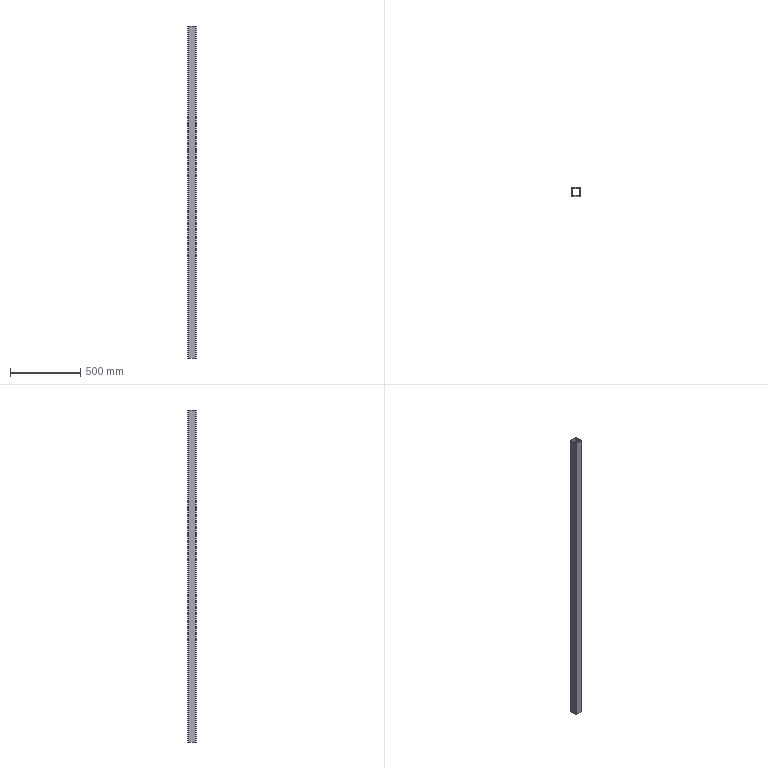Part | STEP file | 750078154 | 1 solid | 18 faces | box 60 x 60 x 2360 mm | volume 2049733 mm3 | plane 10 | cylinder 8 | commonest cylinder face diameters 4 x4 12 x4
STEP:
#1=CARTESIAN_POINT('',(-26.,24.,2360.));
#2=VERTEX_POINT('',#1);
#3=CARTESIAN_POINT('',(-26.,24.,0.));
#4=VERTEX_POINT('',#3);
#5=CARTESIAN_POINT('',(-26.,24.,2360.));
#6=DIRECTION('',(0.,0.,-1.));
#7=VECTOR('',#6,1000.);
#8=LINE('',#5,#7);
#9=EDGE_CURVE('',#2,#4,#8,.T.);
#10=ORIENTED_EDGE('',*,*,#9,.F.);
#11=CARTESIAN_POINT('',(-26.,-24.,2360.));
#12=VERTEX_POINT('',#11);
#13=CARTESIAN_POINT('',(-26.,-24.,2360.));
#14=DIRECTION('',(0.,1.,0.));
#15=VECTOR('',#14,1000.);
#16=LINE('',#13,#15);
#17=EDGE_CURVE('',#12,#2,#16,.T.);
#18=ORIENTED_EDGE('',*,*,#17,.F.);
#19=CARTESIAN_POINT('',(-26.,-24.,0.));
#20=VERTEX_POINT('',#19);
#21=CARTESIAN_POINT('',(-26.,-24.,2360.));
#22=DIRECTION('',(0.,0.,1.));
#23=VECTOR('',#22,1000.);
#24=LINE('',#21,#23);
#25=EDGE_CURVE('',#20,#12,#24,.T.);
#26=ORIENTED_EDGE('',*,*,#25,.F.);
#27=CARTESIAN_POINT('',(-26.,-24.,0.));
#28=DIRECTION('',(0.,-1.,0.));
#29=VECTOR('',#28,1000.);
#30=LINE('',#27,#29);
#31=EDGE_CURVE('',#4,#20,#30,.T.);
#32=ORIENTED_EDGE('',*,*,#31,.F.);
#33=EDGE_LOOP('',(#10,#18,#26,#32));
#34=FACE_OUTER_BOUND('',#33,.T.);
#35=CARTESIAN_POINT('',(-26.,-24.,2360.));
#36=DIRECTION('',(-1.,0.,0.));
#37=DIRECTION('',(0.,-1.,0.));
#38=AXIS2_PLACEMENT_3D('',#35,#36,#37);
#39=PLANE('',#38);
#40=ADVANCED_FACE('',(#34),#39,.F.);
#41=CARTESIAN_POINT('',(26.,24.,0.));
#42=VERTEX_POINT('',#41);
#43=CARTESIAN_POINT('',(24.,26.,0.));
#44=VERTEX_POINT('',#43);
#45=CARTESIAN_POINT('',(24.,24.,0.));
#46=DIRECTION('',(0.,0.,1.));
#47=DIRECTION('',(-1.,0.,0.));
#48=AXIS2_PLACEMENT_3D('',#45,#46,#47);
#49=CIRCLE('',#48,2.);
#50=EDGE_CURVE('',#42,#44,#49,.T.);
#51=ORIENTED_EDGE('',*,*,#50,.T.);
#52=CARTESIAN_POINT('',(-24.,26.,0.));
#53=VERTEX_POINT('',#52);
#54=CARTESIAN_POINT('',(24.,26.,0.));
#55=DIRECTION('',(-1.,0.,0.));
#56=VECTOR('',#55,1000.);
#57=LINE('',#54,#56);
#58=EDGE_CURVE('',#44,#53,#57,.T.);
#59=ORIENTED_EDGE('',*,*,#58,.T.);
#60=CARTESIAN_POINT('',(-24.,24.,0.));
#61=DIRECTION('',(0.,0.,1.));
#62=DIRECTION('',(-1.,0.,0.));
#63=AXIS2_PLACEMENT_3D('',#60,#61,#62);
#64=CIRCLE('',#63,2.);
#65=EDGE_CURVE('',#53,#4,#64,.T.);
#66=ORIENTED_EDGE('',*,*,#65,.T.);
#67=ORIENTED_EDGE('',*,*,#31,.T.);
#68=CARTESIAN_POINT('',(-24.,-26.,0.));
#69=VERTEX_POINT('',#68);
#70=CARTESIAN_POINT('',(-24.,-24.,0.));
#71=DIRECTION('',(0.,0.,1.));
#72=DIRECTION('',(-1.,0.,0.));
#73=AXIS2_PLACEMENT_3D('',#70,#71,#72);
#74=CIRCLE('',#73,2.);
#75=EDGE_CURVE('',#20,#69,#74,.T.);
#76=ORIENTED_EDGE('',*,*,#75,.T.);
#77=CARTESIAN_POINT('',(24.,-26.,0.));
#78=VERTEX_POINT('',#77);
#79=CARTESIAN_POINT('',(24.,-26.,0.));
#80=DIRECTION('',(1.,0.,0.));
#81=VECTOR('',#80,1000.);
#82=LINE('',#79,#81);
#83=EDGE_CURVE('',#69,#78,#82,.T.);
#84=ORIENTED_EDGE('',*,*,#83,.T.);
#85=CARTESIAN_POINT('',(26.,-24.,0.));
#86=VERTEX_POINT('',#85);
#87=CARTESIAN_POINT('',(24.,-24.,0.));
#88=DIRECTION('',(0.,0.,1.));
#89=DIRECTION('',(-1.,0.,0.));
#90=AXIS2_PLACEMENT_3D('',#87,#88,#89);
#91=CIRCLE('',#90,2.);
#92=EDGE_CURVE('',#78,#86,#91,.T.);
#93=ORIENTED_EDGE('',*,*,#92,.T.);
#94=CARTESIAN_POINT('',(26.,-24.,0.));
#95=DIRECTION('',(0.,1.,0.));
#96=VECTOR('',#95,1000.);
#97=LINE('',#94,#96);
#98=EDGE_CURVE('',#86,#42,#97,.T.);
#99=ORIENTED_EDGE('',*,*,#98,.T.);
#100=EDGE_LOOP('',(#51,#59,#66,#67,#76,#84,#93,#99));
#101=FACE_BOUND('',#100,.T.);
#102=CARTESIAN_POINT('',(-24.,30.,0.));
#103=VERTEX_POINT('',#102);
#104=CARTESIAN_POINT('',(24.,30.,0.));
#105=VERTEX_POINT('',#104);
#106=CARTESIAN_POINT('',(24.,30.,0.));
#107=DIRECTION('',(1.,0.,0.));
#108=VECTOR('',#107,1000.);
#109=LINE('',#106,#108);
#110=EDGE_CURVE('',#103,#105,#109,.T.);
#111=ORIENTED_EDGE('',*,*,#110,.T.);
#112=CARTESIAN_POINT('',(30.,24.,0.));
#113=VERTEX_POINT('',#112);
#114=CARTESIAN_POINT('',(24.,24.,0.));
#115=DIRECTION('',(0.,0.,-1.));
#116=DIRECTION('',(-1.,0.,0.));
#117=AXIS2_PLACEMENT_3D('',#114,#115,#116);
#118=CIRCLE('',#117,6.);
#119=EDGE_CURVE('',#105,#113,#118,.T.);
#120=ORIENTED_EDGE('',*,*,#119,.T.);
#121=CARTESIAN_POINT('',(30.,-24.,0.));
#122=VERTEX_POINT('',#121);
#123=CARTESIAN_POINT('',(30.,-24.,0.));
#124=DIRECTION('',(0.,-1.,0.));
#125=VECTOR('',#124,1000.);
#126=LINE('',#123,#125);
#127=EDGE_CURVE('',#113,#122,#126,.T.);
#128=ORIENTED_EDGE('',*,*,#127,.T.);
#129=CARTESIAN_POINT('',(24.,-30.,0.));
#130=VERTEX_POINT('',#129);
#131=CARTESIAN_POINT('',(24.,-24.,0.));
#132=DIRECTION('',(0.,0.,-1.));
#133=DIRECTION('',(-1.,0.,0.));
#134=AXIS2_PLACEMENT_3D('',#131,#132,#133);
#135=CIRCLE('',#134,6.);
#136=EDGE_CURVE('',#122,#130,#135,.T.);
#137=ORIENTED_EDGE('',*,*,#136,.T.);
#138=CARTESIAN_POINT('',(-24.,-30.,0.));
#139=VERTEX_POINT('',#138);
#140=CARTESIAN_POINT('',(24.,-30.,0.));
#141=DIRECTION('',(-1.,0.,0.));
#142=VECTOR('',#141,1000.);
#143=LINE('',#140,#142);
#144=EDGE_CURVE('',#130,#139,#143,.T.);
#145=ORIENTED_EDGE('',*,*,#144,.T.);
#146=CARTESIAN_POINT('',(-30.,-24.,0.));
#147=VERTEX_POINT('',#146);
#148=CARTESIAN_POINT('',(-24.,-24.,0.));
#149=DIRECTION('',(0.,0.,-1.));
#150=DIRECTION('',(-1.,0.,0.));
#151=AXIS2_PLACEMENT_3D('',#148,#149,#150);
#152=CIRCLE('',#151,6.);
#153=EDGE_CURVE('',#139,#147,#152,.T.);
#154=ORIENTED_EDGE('',*,*,#153,.T.);
#155=CARTESIAN_POINT('',(-30.,24.,0.));
#156=VERTEX_POINT('',#155);
#157=CARTESIAN_POINT('',(-30.,-24.,0.));
#158=DIRECTION('',(0.,1.,0.));
#159=VECTOR('',#158,1000.);
#160=LINE('',#157,#159);
#161=EDGE_CURVE('',#147,#156,#160,.T.);
#162=ORIENTED_EDGE('',*,*,#161,.T.);
#163=CARTESIAN_POINT('',(-24.,24.,0.));
#164=DIRECTION('',(0.,0.,-1.));
#165=DIRECTION('',(-1.,0.,0.));
#166=AXIS2_PLACEMENT_3D('',#163,#164,#165);
#167=CIRCLE('',#166,6.);
#168=EDGE_CURVE('',#156,#103,#167,.T.);
#169=ORIENTED_EDGE('',*,*,#168,.T.);
#170=EDGE_LOOP('',(#111,#120,#128,#137,#145,#154,#162,#169));
#171=FACE_OUTER_BOUND('',#170,.T.);
#172=CARTESIAN_POINT('',(24.,-24.,0.));
#173=DIRECTION('',(0.,0.,-1.));
#174=DIRECTION('',(-1.,0.,0.));
#175=AXIS2_PLACEMENT_3D('',#172,#173,#174);
#176=PLANE('',#175);
#177=ADVANCED_FACE('',(#101,#171),#176,.T.);
#178=CARTESIAN_POINT('',(-24.,26.,2360.));
#179=VERTEX_POINT('',#178);
#180=CARTESIAN_POINT('',(-24.,26.,2360.));
#181=DIRECTION('',(0.,0.,-1.));
#182=VECTOR('',#181,1000.);
#183=LINE('',#180,#182);
#184=EDGE_CURVE('',#179,#53,#183,.T.);
#185=ORIENTED_EDGE('',*,*,#184,.F.);
#186=CARTESIAN_POINT('',(-24.,24.,2360.));
#187=DIRECTION('',(0.,0.,-1.));
#188=DIRECTION('',(-1.,0.,0.));
#189=AXIS2_PLACEMENT_3D('',#186,#187,#188);
#190=CIRCLE('',#189,2.);
#191=EDGE_CURVE('',#2,#179,#190,.T.);
#192=ORIENTED_EDGE('',*,*,#191,.F.);
#193=ORIENTED_EDGE('',*,*,#9,.T.);
#194=ORIENTED_EDGE('',*,*,#65,.F.);
#195=EDGE_LOOP('',(#185,#192,#193,#194));
#196=FACE_OUTER_BOUND('',#195,.T.);
#197=CARTESIAN_POINT('',(-24.,24.,2360.));
#198=DIRECTION('',(0.,0.,-1.));
#199=DIRECTION('',(-1.,0.,0.));
#200=AXIS2_PLACEMENT_3D('',#197,#198,#199);
#201=CYLINDRICAL_SURFACE('',#200,2.);
#202=ADVANCED_FACE('',(#196),#201,.F.);
#203=CARTESIAN_POINT('',(24.,26.,2360.));
#204=VERTEX_POINT('',#203);
#205=CARTESIAN_POINT('',(24.,26.,2360.));
#206=DIRECTION('',(-1.,0.,0.));
#207=VECTOR('',#206,1000.);
#208=LINE('',#205,#207);
#209=EDGE_CURVE('',#204,#179,#208,.T.);
#210=ORIENTED_EDGE('',*,*,#209,.F.);
#211=CARTESIAN_POINT('',(26.,24.,2360.));
#212=VERTEX_POINT('',#211);
#213=CARTESIAN_POINT('',(24.,24.,2360.));
#214=DIRECTION('',(0.,0.,1.));
#215=DIRECTION('',(-1.,0.,0.));
#216=AXIS2_PLACEMENT_3D('',#213,#214,#215);
#217=CIRCLE('',#216,2.);
#218=EDGE_CURVE('',#212,#204,#217,.T.);
#219=ORIENTED_EDGE('',*,*,#218,.F.);
#220=CARTESIAN_POINT('',(26.,-24.,2360.));
#221=VERTEX_POINT('',#220);
#222=CARTESIAN_POINT('',(26.,-24.,2360.));
#223=DIRECTION('',(0.,1.,0.));
#224=VECTOR('',#223,1000.);
#225=LINE('',#222,#224);
#226=EDGE_CURVE('',#221,#212,#225,.T.);
#227=ORIENTED_EDGE('',*,*,#226,.F.);
#228=CARTESIAN_POINT('',(24.,-26.,2360.));
#229=VERTEX_POINT('',#228);
#230=CARTESIAN_POINT('',(24.,-24.,2360.));
#231=DIRECTION('',(0.,0.,1.));
#232=DIRECTION('',(-1.,0.,0.));
#233=AXIS2_PLACEMENT_3D('',#230,#231,#232);
#234=CIRCLE('',#233,2.);
#235=EDGE_CURVE('',#229,#221,#234,.T.);
#236=ORIENTED_EDGE('',*,*,#235,.F.);
#237=CARTESIAN_POINT('',(-24.,-26.,2360.));
#238=VERTEX_POINT('',#237);
#239=CARTESIAN_POINT('',(24.,-26.,2360.));
#240=DIRECTION('',(1.,0.,0.));
#241=VECTOR('',#240,1000.);
#242=LINE('',#239,#241);
#243=EDGE_CURVE('',#238,#229,#242,.T.);
#244=ORIENTED_EDGE('',*,*,#243,.F.);
#245=CARTESIAN_POINT('',(-24.,-24.,2360.));
#246=DIRECTION('',(0.,0.,1.));
#247=DIRECTION('',(-1.,0.,0.));
#248=AXIS2_PLACEMENT_3D('',#245,#246,#247);
#249=CIRCLE('',#248,2.);
#250=EDGE_CURVE('',#12,#238,#249,.T.);
#251=ORIENTED_EDGE('',*,*,#250,.F.);
#252=ORIENTED_EDGE('',*,*,#17,.T.);
#253=ORIENTED_EDGE('',*,*,#191,.T.);
#254=EDGE_LOOP('',(#210,#219,#227,#236,#244,#251,#252,#253));
#255=FACE_BOUND('',#254,.T.);
#256=CARTESIAN_POINT('',(24.,30.,2360.));
#257=VERTEX_POINT('',#256);
#258=CARTESIAN_POINT('',(30.,24.,2360.));
#259=VERTEX_POINT('',#258);
#260=CARTESIAN_POINT('',(24.,24.,2360.));
#261=DIRECTION('',(0.,0.,-1.));
#262=DIRECTION('',(-1.,0.,0.));
#263=AXIS2_PLACEMENT_3D('',#260,#261,#262);
#264=CIRCLE('',#263,6.);
#265=EDGE_CURVE('',#257,#259,#264,.T.);
#266=ORIENTED_EDGE('',*,*,#265,.F.);
#267=CARTESIAN_POINT('',(-24.,30.,2360.));
#268=VERTEX_POINT('',#267);
#269=CARTESIAN_POINT('',(24.,30.,2360.));
#270=DIRECTION('',(1.,0.,0.));
#271=VECTOR('',#270,1000.);
#272=LINE('',#269,#271);
#273=EDGE_CURVE('',#268,#257,#272,.T.);
#274=ORIENTED_EDGE('',*,*,#273,.F.);
#275=CARTESIAN_POINT('',(-30.,24.,2360.));
#276=VERTEX_POINT('',#275);
#277=CARTESIAN_POINT('',(-24.,24.,2360.));
#278=DIRECTION('',(0.,0.,-1.));
#279=DIRECTION('',(-1.,0.,0.));
#280=AXIS2_PLACEMENT_3D('',#277,#278,#279);
#281=CIRCLE('',#280,6.);
#282=EDGE_CURVE('',#276,#268,#281,.T.);
#283=ORIENTED_EDGE('',*,*,#282,.F.);
#284=CARTESIAN_POINT('',(-30.,-24.,2360.));
#285=VERTEX_POINT('',#284);
#286=CARTESIAN_POINT('',(-30.,-24.,2360.));
#287=DIRECTION('',(0.,1.,0.));
#288=VECTOR('',#287,1000.);
#289=LINE('',#286,#288);
#290=EDGE_CURVE('',#285,#276,#289,.T.);
#291=ORIENTED_EDGE('',*,*,#290,.F.);
#292=CARTESIAN_POINT('',(-24.,-30.,2360.));
#293=VERTEX_POINT('',#292);
#294=CARTESIAN_POINT('',(-24.,-24.,2360.));
#295=DIRECTION('',(0.,0.,-1.));
#296=DIRECTION('',(-1.,0.,0.));
#297=AXIS2_PLACEMENT_3D('',#294,#295,#296);
#298=CIRCLE('',#297,6.);
#299=EDGE_CURVE('',#293,#285,#298,.T.);
#300=ORIENTED_EDGE('',*,*,#299,.F.);
#301=CARTESIAN_POINT('',(24.,-30.,2360.));
#302=VERTEX_POINT('',#301);
#303=CARTESIAN_POINT('',(24.,-30.,2360.));
#304=DIRECTION('',(-1.,0.,0.));
#305=VECTOR('',#304,1000.);
#306=LINE('',#303,#305);
#307=EDGE_CURVE('',#302,#293,#306,.T.);
#308=ORIENTED_EDGE('',*,*,#307,.F.);
#309=CARTESIAN_POINT('',(30.,-24.,2360.));
#310=VERTEX_POINT('',#309);
#311=CARTESIAN_POINT('',(24.,-24.,2360.));
#312=DIRECTION('',(0.,0.,-1.));
#313=DIRECTION('',(-1.,0.,0.));
#314=AXIS2_PLACEMENT_3D('',#311,#312,#313);
#315=CIRCLE('',#314,6.);
#316=EDGE_CURVE('',#310,#302,#315,.T.);
#317=ORIENTED_EDGE('',*,*,#316,.F.);
#318=CARTESIAN_POINT('',(30.,-24.,2360.));
#319=DIRECTION('',(0.,-1.,0.));
#320=VECTOR('',#319,1000.);
#321=LINE('',#318,#320);
#322=EDGE_CURVE('',#259,#310,#321,.T.);
#323=ORIENTED_EDGE('',*,*,#322,.F.);
#324=EDGE_LOOP('',(#266,#274,#283,#291,#300,#308,#317,#323));
#325=FACE_OUTER_BOUND('',#324,.T.);
#326=CARTESIAN_POINT('',(24.,-24.,2360.));
#327=DIRECTION('',(0.,0.,-1.));
#328=DIRECTION('',(-1.,0.,0.));
#329=AXIS2_PLACEMENT_3D('',#326,#327,#328);
#330=PLANE('',#329);
#331=ADVANCED_FACE('',(#255,#325),#330,.F.);
#332=ORIENTED_EDGE('',*,*,#25,.T.);
#333=ORIENTED_EDGE('',*,*,#250,.T.);
#334=CARTESIAN_POINT('',(-24.,-26.,2360.));
#335=DIRECTION('',(0.,0.,1.));
#336=VECTOR('',#335,1000.);
#337=LINE('',#334,#336);
#338=EDGE_CURVE('',#69,#238,#337,.T.);
#339=ORIENTED_EDGE('',*,*,#338,.F.);
#340=ORIENTED_EDGE('',*,*,#75,.F.);
#341=EDGE_LOOP('',(#332,#333,#339,#340));
#342=FACE_OUTER_BOUND('',#341,.T.);
#343=CARTESIAN_POINT('',(-24.,-24.,2360.));
#344=DIRECTION('',(0.,0.,-1.));
#345=DIRECTION('',(-1.,0.,0.));
#346=AXIS2_PLACEMENT_3D('',#343,#344,#345);
#347=CYLINDRICAL_SURFACE('',#346,2.);
#348=ADVANCED_FACE('',(#342),#347,.F.);
#349=CARTESIAN_POINT('',(24.,26.,2360.));
#350=DIRECTION('',(0.,0.,-1.));
#351=VECTOR('',#350,1000.);
#352=LINE('',#349,#351);
#353=EDGE_CURVE('',#204,#44,#352,.T.);
#354=ORIENTED_EDGE('',*,*,#353,.F.);
#355=ORIENTED_EDGE('',*,*,#209,.T.);
#356=ORIENTED_EDGE('',*,*,#184,.T.);
#357=ORIENTED_EDGE('',*,*,#58,.F.);
#358=EDGE_LOOP('',(#354,#355,#356,#357));
#359=FACE_OUTER_BOUND('',#358,.T.);
#360=CARTESIAN_POINT('',(-24.,26.,2360.));
#361=DIRECTION('',(0.,1.,0.));
#362=DIRECTION('',(0.,0.,1.));
#363=AXIS2_PLACEMENT_3D('',#360,#361,#362);
#364=PLANE('',#363);
#365=ADVANCED_FACE('',(#359),#364,.F.);
#366=CARTESIAN_POINT('',(26.,24.,2360.));
#367=DIRECTION('',(0.,0.,-1.));
#368=VECTOR('',#367,1000.);
#369=LINE('',#366,#368);
#370=EDGE_CURVE('',#212,#42,#369,.T.);
#371=ORIENTED_EDGE('',*,*,#370,.F.);
#372=ORIENTED_EDGE('',*,*,#218,.T.);
#373=ORIENTED_EDGE('',*,*,#353,.T.);
#374=ORIENTED_EDGE('',*,*,#50,.F.);
#375=EDGE_LOOP('',(#371,#372,#373,#374));
#376=FACE_OUTER_BOUND('',#375,.T.);
#377=CARTESIAN_POINT('',(24.,24.,2360.));
#378=DIRECTION('',(0.,0.,-1.));
#379=DIRECTION('',(-1.,0.,0.));
#380=AXIS2_PLACEMENT_3D('',#377,#378,#379);
#381=CYLINDRICAL_SURFACE('',#380,2.);
#382=ADVANCED_FACE('',(#376),#381,.F.);
#383=CARTESIAN_POINT('',(26.,-24.,2360.));
#384=DIRECTION('',(0.,0.,-1.));
#385=VECTOR('',#384,1000.);
#386=LINE('',#383,#385);
#387=EDGE_CURVE('',#221,#86,#386,.T.);
#388=ORIENTED_EDGE('',*,*,#387,.F.);
#389=ORIENTED_EDGE('',*,*,#226,.T.);
#390=ORIENTED_EDGE('',*,*,#370,.T.);
#391=ORIENTED_EDGE('',*,*,#98,.F.);
#392=EDGE_LOOP('',(#388,#389,#390,#391));
#393=FACE_OUTER_BOUND('',#392,.T.);
#394=CARTESIAN_POINT('',(26.,24.,2360.));
#395=DIRECTION('',(1.,0.,0.));
#396=DIRECTION('',(0.,0.,-1.));
#397=AXIS2_PLACEMENT_3D('',#394,#395,#396);
#398=PLANE('',#397);
#399=ADVANCED_FACE('',(#393),#398,.F.);
#400=CARTESIAN_POINT('',(24.,-26.,2360.));
#401=DIRECTION('',(0.,0.,-1.));
#402=VECTOR('',#401,1000.);
#403=LINE('',#400,#402);
#404=EDGE_CURVE('',#229,#78,#403,.T.);
#405=ORIENTED_EDGE('',*,*,#404,.F.);
#406=ORIENTED_EDGE('',*,*,#235,.T.);
#407=ORIENTED_EDGE('',*,*,#387,.T.);
#408=ORIENTED_EDGE('',*,*,#92,.F.);
#409=EDGE_LOOP('',(#405,#406,#407,#408));
#410=FACE_OUTER_BOUND('',#409,.T.);
#411=CARTESIAN_POINT('',(24.,-24.,2360.));
#412=DIRECTION('',(0.,0.,-1.));
#413=DIRECTION('',(-1.,0.,0.));
#414=AXIS2_PLACEMENT_3D('',#411,#412,#413);
#415=CYLINDRICAL_SURFACE('',#414,2.);
#416=ADVANCED_FACE('',(#410),#415,.F.);
#417=ORIENTED_EDGE('',*,*,#338,.T.);
#418=ORIENTED_EDGE('',*,*,#243,.T.);
#419=ORIENTED_EDGE('',*,*,#404,.T.);
#420=ORIENTED_EDGE('',*,*,#83,.F.);
#421=EDGE_LOOP('',(#417,#418,#419,#420));
#422=FACE_OUTER_BOUND('',#421,.T.);
#423=CARTESIAN_POINT('',(24.,-26.,2360.));
#424=DIRECTION('',(0.,-1.,0.));
#425=DIRECTION('',(0.,0.,-1.));
#426=AXIS2_PLACEMENT_3D('',#423,#424,#425);
#427=PLANE('',#426);
#428=ADVANCED_FACE('',(#422),#427,.F.);
#429=ORIENTED_EDGE('',*,*,#265,.T.);
#430=CARTESIAN_POINT('',(30.,24.,2360.));
#431=DIRECTION('',(0.,0.,-1.));
#432=VECTOR('',#431,1000.);
#433=LINE('',#430,#432);
#434=EDGE_CURVE('',#259,#113,#433,.T.);
#435=ORIENTED_EDGE('',*,*,#434,.T.);
#436=ORIENTED_EDGE('',*,*,#119,.F.);
#437=CARTESIAN_POINT('',(24.,30.,2360.));
#438=DIRECTION('',(0.,0.,1.));
#439=VECTOR('',#438,1000.);
#440=LINE('',#437,#439);
#441=EDGE_CURVE('',#105,#257,#440,.T.);
#442=ORIENTED_EDGE('',*,*,#441,.T.);
#443=EDGE_LOOP('',(#429,#435,#436,#442));
#444=FACE_OUTER_BOUND('',#443,.T.);
#445=CARTESIAN_POINT('',(24.,24.,2360.));
#446=DIRECTION('',(0.,0.,-1.));
#447=DIRECTION('',(-1.,0.,0.));
#448=AXIS2_PLACEMENT_3D('',#445,#446,#447);
#449=CYLINDRICAL_SURFACE('',#448,6.);
#450=ADVANCED_FACE('',(#444),#449,.T.);
#451=ORIENTED_EDGE('',*,*,#273,.T.);
#452=ORIENTED_EDGE('',*,*,#441,.F.);
#453=ORIENTED_EDGE('',*,*,#110,.F.);
#454=CARTESIAN_POINT('',(-24.,30.,2360.));
#455=DIRECTION('',(0.,0.,1.));
#456=VECTOR('',#455,1000.);
#457=LINE('',#454,#456);
#458=EDGE_CURVE('',#103,#268,#457,.T.);
#459=ORIENTED_EDGE('',*,*,#458,.T.);
#460=EDGE_LOOP('',(#451,#452,#453,#459));
#461=FACE_OUTER_BOUND('',#460,.T.);
#462=CARTESIAN_POINT('',(-24.,30.,2360.));
#463=DIRECTION('',(0.,1.,0.));
#464=DIRECTION('',(-1.,0.,0.));
#465=AXIS2_PLACEMENT_3D('',#462,#463,#464);
#466=PLANE('',#465);
#467=ADVANCED_FACE('',(#461),#466,.T.);
#468=ORIENTED_EDGE('',*,*,#282,.T.);
#469=ORIENTED_EDGE('',*,*,#458,.F.);
#470=ORIENTED_EDGE('',*,*,#168,.F.);
#471=CARTESIAN_POINT('',(-30.,24.,2360.));
#472=DIRECTION('',(0.,0.,1.));
#473=VECTOR('',#472,1000.);
#474=LINE('',#471,#473);
#475=EDGE_CURVE('',#156,#276,#474,.T.);
#476=ORIENTED_EDGE('',*,*,#475,.T.);
#477=EDGE_LOOP('',(#468,#469,#470,#476));
#478=FACE_OUTER_BOUND('',#477,.T.);
#479=CARTESIAN_POINT('',(-24.,24.,2360.));
#480=DIRECTION('',(0.,0.,-1.));
#481=DIRECTION('',(-1.,0.,0.));
#482=AXIS2_PLACEMENT_3D('',#479,#480,#481);
#483=CYLINDRICAL_SURFACE('',#482,6.);
#484=ADVANCED_FACE('',(#478),#483,.T.);
#485=ORIENTED_EDGE('',*,*,#290,.T.);
#486=ORIENTED_EDGE('',*,*,#475,.F.);
#487=ORIENTED_EDGE('',*,*,#161,.F.);
#488=CARTESIAN_POINT('',(-30.,-24.,2360.));
#489=DIRECTION('',(0.,0.,1.));
#490=VECTOR('',#489,1000.);
#491=LINE('',#488,#490);
#492=EDGE_CURVE('',#147,#285,#491,.T.);
#493=ORIENTED_EDGE('',*,*,#492,.T.);
#494=EDGE_LOOP('',(#485,#486,#487,#493));
#495=FACE_OUTER_BOUND('',#494,.T.);
#496=CARTESIAN_POINT('',(-30.,-24.,2360.));
#497=DIRECTION('',(-1.,0.,0.));
#498=DIRECTION('',(0.,-1.,0.));
#499=AXIS2_PLACEMENT_3D('',#496,#497,#498);
#500=PLANE('',#499);
#501=ADVANCED_FACE('',(#495),#500,.T.);
#502=ORIENTED_EDGE('',*,*,#299,.T.);
#503=ORIENTED_EDGE('',*,*,#492,.F.);
#504=ORIENTED_EDGE('',*,*,#153,.F.);
#505=CARTESIAN_POINT('',(-24.,-30.,2360.));
#506=DIRECTION('',(0.,0.,1.));
#507=VECTOR('',#506,1000.);
#508=LINE('',#505,#507);
#509=EDGE_CURVE('',#139,#293,#508,.T.);
#510=ORIENTED_EDGE('',*,*,#509,.T.);
#511=EDGE_LOOP('',(#502,#503,#504,#510));
#512=FACE_OUTER_BOUND('',#511,.T.);
#513=CARTESIAN_POINT('',(-24.,-24.,2360.));
#514=DIRECTION('',(0.,0.,-1.));
#515=DIRECTION('',(-1.,0.,0.));
#516=AXIS2_PLACEMENT_3D('',#513,#514,#515);
#517=CYLINDRICAL_SURFACE('',#516,6.);
#518=ADVANCED_FACE('',(#512),#517,.T.);
#519=ORIENTED_EDGE('',*,*,#307,.T.);
#520=ORIENTED_EDGE('',*,*,#509,.F.);
#521=ORIENTED_EDGE('',*,*,#144,.F.);
#522=CARTESIAN_POINT('',(24.,-30.,2360.));
#523=DIRECTION('',(0.,0.,1.));
#524=VECTOR('',#523,1000.);
#525=LINE('',#522,#524);
#526=EDGE_CURVE('',#130,#302,#525,.T.);
#527=ORIENTED_EDGE('',*,*,#526,.T.);
#528=EDGE_LOOP('',(#519,#520,#521,#527));
#529=FACE_OUTER_BOUND('',#528,.T.);
#530=CARTESIAN_POINT('',(24.,-30.,2360.));
#531=DIRECTION('',(0.,-1.,0.));
#532=DIRECTION('',(1.,0.,0.));
#533=AXIS2_PLACEMENT_3D('',#530,#531,#532);
#534=PLANE('',#533);
#535=ADVANCED_FACE('',(#529),#534,.T.);
#536=ORIENTED_EDGE('',*,*,#316,.T.);
#537=ORIENTED_EDGE('',*,*,#526,.F.);
#538=ORIENTED_EDGE('',*,*,#136,.F.);
#539=CARTESIAN_POINT('',(30.,-24.,2360.));
#540=DIRECTION('',(0.,0.,1.));
#541=VECTOR('',#540,1000.);
#542=LINE('',#539,#541);
#543=EDGE_CURVE('',#122,#310,#542,.T.);
#544=ORIENTED_EDGE('',*,*,#543,.T.);
#545=EDGE_LOOP('',(#536,#537,#538,#544));
#546=FACE_OUTER_BOUND('',#545,.T.);
#547=CARTESIAN_POINT('',(24.,-24.,2360.));
#548=DIRECTION('',(0.,0.,-1.));
#549=DIRECTION('',(-1.,0.,0.));
#550=AXIS2_PLACEMENT_3D('',#547,#548,#549);
#551=CYLINDRICAL_SURFACE('',#550,6.);
#552=ADVANCED_FACE('',(#546),#551,.T.);
#553=ORIENTED_EDGE('',*,*,#322,.T.);
#554=ORIENTED_EDGE('',*,*,#543,.F.);
#555=ORIENTED_EDGE('',*,*,#127,.F.);
#556=ORIENTED_EDGE('',*,*,#434,.F.);
#557=EDGE_LOOP('',(#553,#554,#555,#556));
#558=FACE_OUTER_BOUND('',#557,.T.);
#559=CARTESIAN_POINT('',(30.,24.,2360.));
#560=DIRECTION('',(1.,0.,0.));
#561=DIRECTION('',(0.,0.,-1.));
#562=AXIS2_PLACEMENT_3D('',#559,#560,#561);
#563=PLANE('',#562);
#564=ADVANCED_FACE('',(#558),#563,.T.);
#565=CLOSED_SHELL('',(#40,#177,#202,#331,#348,#365,#382,#399,#416,#428,#450,#467,#484,#501,#518,#535,#552,#564));
#566=MANIFOLD_SOLID_BREP('',#565);
#567=CARTESIAN_POINT('',(0.,0.,0.));
#568=DIRECTION('',(0.,0.,1.));
#569=DIRECTION('',(1.,0.,0.));
#570=AXIS2_PLACEMENT_3D('',#567,#568,#569);
#571=(LENGTH_UNIT()NAMED_UNIT(*)SI_UNIT(.MILLI.,.METRE.));
#572=UNCERTAINTY_MEASURE_WITH_UNIT(LENGTH_MEASURE(0.00001),#571,'','');
#573=(NAMED_UNIT(*)PLANE_ANGLE_UNIT()SI_UNIT($,.RADIAN.));
#574=(NAMED_UNIT(*)SI_UNIT($,.STERADIAN.)SOLID_ANGLE_UNIT());
#575=(GEOMETRIC_REPRESENTATION_CONTEXT(3)GLOBAL_UNCERTAINTY_ASSIGNED_CONTEXT((#572))GLOBAL_UNIT_ASSIGNED_CONTEXT((#571,#573,#574))REPRESENTATION_CONTEXT('',''));
#576=ADVANCED_BREP_SHAPE_REPRESENTATION('',(#566,#570),#575);